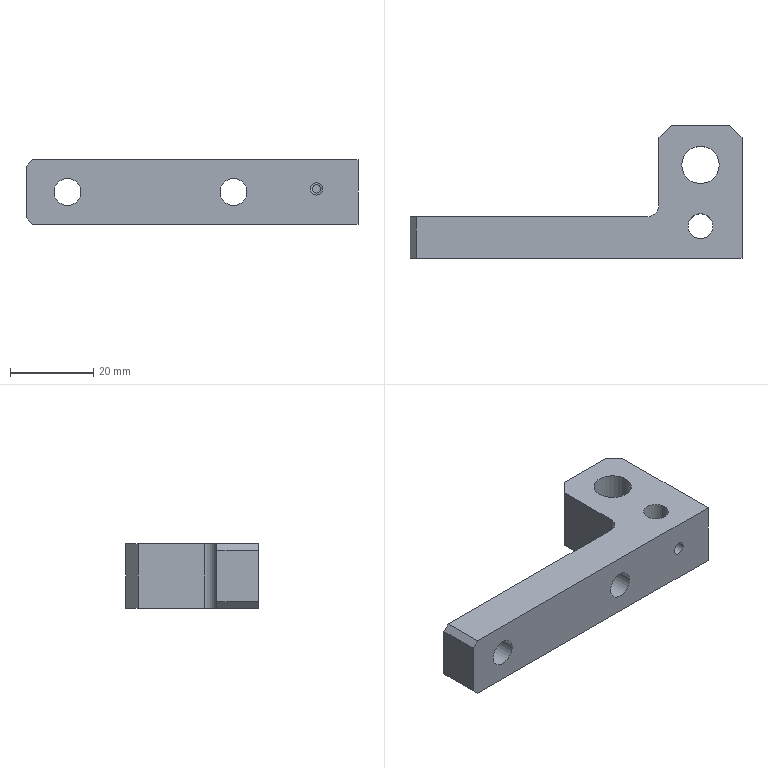Part | NX | 1 solid | 21 faces | box 80 x 32 x 15.5 mm | volume 16646 mm3 | plane 13 | cylinder 8 | commonest cylinder face diameters 6 x2 6.5 x2 2 x1 3 x1 9 x1 12 x1
STEP:
#1=CARTESIAN_POINT('',(70.,18.,9.5));
#2=VERTEX_POINT('',#1);
#3=CARTESIAN_POINT('',(70.784,18.056,9.283));
#4=CARTESIAN_POINT('',(70.,17.972,9.609));
#5=CARTESIAN_POINT('',(69.216,18.056,9.283));
#6=CARTESIAN_POINT('',(68.892,18.141,8.501));
#7=CARTESIAN_POINT('',(69.216,18.056,7.716));
#8=CARTESIAN_POINT('',(70.,17.972,7.392));
#9=CARTESIAN_POINT('',(70.783,18.055,7.716));
#10=CARTESIAN_POINT('',(71.108,18.141,8.499));
#11=CARTESIAN_POINT('',(70.784,18.056,9.283));
#12=CARTESIAN_POINT('',(70.,17.972,9.609));
#13=CARTESIAN_POINT('',(69.216,18.056,9.283));
#14=B_SPLINE_CURVE_WITH_KNOTS('',3,(#3,#4,#5,#6,#7,#8,#9,#10,#11,#12,#13),.UNSPECIFIED.,.T.,.F.,(1,1,1,1,1,1,1,1,1,1,1,1,1,1,1),(-0.002352,-0.001568,-0.000784,0.,0.000784,0.001568,0.002352,0.003136,0.00392,0.004704,0.005488,0.006272,0.007056,0.00784,0.008624),.UNSPECIFIED.);
#15=EDGE_CURVE('',#2,#2,#14,.T.);
#16=ORIENTED_EDGE('',*,*,#15,.T.);
#17=EDGE_LOOP('',(#16));
#18=FACE_BOUND('',#17,.T.);
#19=CARTESIAN_POINT('',(65.5,22.5,15.5));
#20=VERTEX_POINT('',#19);
#21=CARTESIAN_POINT('',(70.,22.5,15.5));
#22=DIRECTION('',(0.,0.,-1.));
#23=DIRECTION('',(-1.,0.,0.));
#24=AXIS2_PLACEMENT_3D('',#21,#22,#23);
#25=CIRCLE('',#24,4.5);
#26=EDGE_CURVE('',#20,#20,#25,.T.);
#27=ORIENTED_EDGE('',*,*,#26,.F.);
#28=EDGE_LOOP('',(#27));
#29=FACE_BOUND('',#28,.T.);
#30=CARTESIAN_POINT('',(65.5,22.5,6.));
#31=VERTEX_POINT('',#30);
#32=CARTESIAN_POINT('',(70.,22.5,6.));
#33=DIRECTION('',(0.,0.,-1.));
#34=DIRECTION('',(-1.,0.,0.));
#35=AXIS2_PLACEMENT_3D('',#32,#33,#34);
#36=CIRCLE('',#35,4.5);
#37=EDGE_CURVE('',#31,#31,#36,.F.);
#38=ORIENTED_EDGE('',*,*,#37,.F.);
#39=EDGE_LOOP('',(#38));
#40=FACE_BOUND('',#39,.T.);
#41=CARTESIAN_POINT('',(70.,22.5,15.5));
#42=DIRECTION('',(0.,0.,-1.));
#43=DIRECTION('',(-1.,0.,0.));
#44=AXIS2_PLACEMENT_3D('',#41,#42,#43);
#45=CYLINDRICAL_SURFACE('',#44,4.5);
#46=ADVANCED_FACE('',(#18,#29,#40),#45,.F.);
#47=ORIENTED_EDGE('',*,*,#26,.T.);
#48=EDGE_LOOP('',(#47));
#49=FACE_BOUND('',#48,.T.);
#50=CARTESIAN_POINT('',(67.,7.75,15.5));
#51=VERTEX_POINT('',#50);
#52=CARTESIAN_POINT('',(70.,7.75,15.5));
#53=DIRECTION('',(0.,0.,-1.));
#54=DIRECTION('',(-1.,0.,0.));
#55=AXIS2_PLACEMENT_3D('',#52,#53,#54);
#56=CIRCLE('',#55,3.);
#57=EDGE_CURVE('',#51,#51,#56,.T.);
#58=ORIENTED_EDGE('',*,*,#57,.T.);
#59=EDGE_LOOP('',(#58));
#60=FACE_BOUND('',#59,.T.);
#61=CARTESIAN_POINT('',(57.,10.,15.5));
#62=VERTEX_POINT('',#61);
#63=CARTESIAN_POINT('',(1.5,10.,15.5));
#64=VERTEX_POINT('',#63);
#65=CARTESIAN_POINT('',(40.,10.,15.5));
#66=DIRECTION('',(-1.,0.,0.));
#67=VECTOR('',#66,1000.);
#68=LINE('',#65,#67);
#69=EDGE_CURVE('',#62,#64,#68,.T.);
#70=ORIENTED_EDGE('',*,*,#69,.T.);
#71=CARTESIAN_POINT('',(1.5,0.,15.5));
#72=VERTEX_POINT('',#71);
#73=CARTESIAN_POINT('',(1.5,16.,15.5));
#74=DIRECTION('',(0.,1.,0.));
#75=VECTOR('',#74,1000.);
#76=LINE('',#73,#75);
#77=EDGE_CURVE('',#64,#72,#76,.F.);
#78=ORIENTED_EDGE('',*,*,#77,.T.);
#79=CARTESIAN_POINT('',(80.,0.,15.5));
#80=VERTEX_POINT('',#79);
#81=CARTESIAN_POINT('',(40.,0.,15.5));
#82=DIRECTION('',(-1.,0.,0.));
#83=VECTOR('',#82,1000.);
#84=LINE('',#81,#83);
#85=EDGE_CURVE('',#80,#72,#84,.T.);
#86=ORIENTED_EDGE('',*,*,#85,.F.);
#87=CARTESIAN_POINT('',(80.,29.,15.5));
#88=VERTEX_POINT('',#87);
#89=CARTESIAN_POINT('',(80.,16.,15.5));
#90=DIRECTION('',(0.,-1.,0.));
#91=VECTOR('',#90,1000.);
#92=LINE('',#89,#91);
#93=EDGE_CURVE('',#88,#80,#92,.T.);
#94=ORIENTED_EDGE('',*,*,#93,.F.);
#95=CARTESIAN_POINT('',(77.,32.,15.5));
#96=VERTEX_POINT('',#95);
#97=CARTESIAN_POINT('',(66.5,42.5,15.5));
#98=DIRECTION('',(0.7071,-0.7071,0.));
#99=VECTOR('',#98,1000.);
#100=LINE('',#97,#99);
#101=EDGE_CURVE('',#88,#96,#100,.F.);
#102=ORIENTED_EDGE('',*,*,#101,.T.);
#103=CARTESIAN_POINT('',(63.,32.,15.5));
#104=VERTEX_POINT('',#103);
#105=CARTESIAN_POINT('',(40.,32.,15.5));
#106=DIRECTION('',(1.,0.,0.));
#107=VECTOR('',#106,1000.);
#108=LINE('',#105,#107);
#109=EDGE_CURVE('',#104,#96,#108,.T.);
#110=ORIENTED_EDGE('',*,*,#109,.F.);
#111=CARTESIAN_POINT('',(60.,29.,15.5));
#112=VERTEX_POINT('',#111);
#113=CARTESIAN_POINT('',(43.5,12.5,15.5));
#114=DIRECTION('',(-0.7071,-0.7071,0.));
#115=VECTOR('',#114,1000.);
#116=LINE('',#113,#115);
#117=EDGE_CURVE('',#104,#112,#116,.T.);
#118=ORIENTED_EDGE('',*,*,#117,.T.);
#119=CARTESIAN_POINT('',(60.,13.,15.5));
#120=VERTEX_POINT('',#119);
#121=CARTESIAN_POINT('',(60.,21.,15.5));
#122=DIRECTION('',(0.,-1.,0.));
#123=VECTOR('',#122,1000.);
#124=LINE('',#121,#123);
#125=EDGE_CURVE('',#112,#120,#124,.T.);
#126=ORIENTED_EDGE('',*,*,#125,.T.);
#127=CARTESIAN_POINT('',(57.,13.,15.5));
#128=DIRECTION('',(0.,0.,1.));
#129=DIRECTION('',(1.,0.,0.));
#130=AXIS2_PLACEMENT_3D('',#127,#128,#129);
#131=CIRCLE('',#130,3.);
#132=EDGE_CURVE('',#120,#62,#131,.F.);
#133=ORIENTED_EDGE('',*,*,#132,.T.);
#134=EDGE_LOOP('',(#70,#78,#86,#94,#102,#110,#118,#126,#133));
#135=FACE_BOUND('',#134,.T.);
#136=CARTESIAN_POINT('',(40.,16.,15.5));
#137=DIRECTION('',(0.,0.,1.));
#138=DIRECTION('',(1.,0.,0.));
#139=AXIS2_PLACEMENT_3D('',#136,#137,#138);
#140=PLANE('',#139);
#141=ADVANCED_FACE('',(#49,#60,#135),#140,.T.);
#142=CARTESIAN_POINT('',(70.,0.,10.));
#143=VERTEX_POINT('',#142);
#144=CARTESIAN_POINT('',(70.,0.,8.5));
#145=DIRECTION('',(0.,1.,0.));
#146=DIRECTION('',(0.,0.,1.));
#147=AXIS2_PLACEMENT_3D('',#144,#145,#146);
#148=CIRCLE('',#147,1.5);
#149=EDGE_CURVE('',#143,#143,#148,.T.);
#150=ORIENTED_EDGE('',*,*,#149,.T.);
#151=EDGE_LOOP('',(#150));
#152=FACE_BOUND('',#151,.T.);
#153=CARTESIAN_POINT('',(50.,0.,11.));
#154=VERTEX_POINT('',#153);
#155=CARTESIAN_POINT('',(50.,0.,7.75));
#156=DIRECTION('',(0.,1.,0.));
#157=DIRECTION('',(0.,0.,1.));
#158=AXIS2_PLACEMENT_3D('',#155,#156,#157);
#159=CIRCLE('',#158,3.25);
#160=EDGE_CURVE('',#154,#154,#159,.T.);
#161=ORIENTED_EDGE('',*,*,#160,.T.);
#162=EDGE_LOOP('',(#161));
#163=FACE_BOUND('',#162,.T.);
#164=CARTESIAN_POINT('',(10.,0.,11.));
#165=VERTEX_POINT('',#164);
#166=CARTESIAN_POINT('',(10.,0.,7.75));
#167=DIRECTION('',(0.,1.,0.));
#168=DIRECTION('',(0.,0.,1.));
#169=AXIS2_PLACEMENT_3D('',#166,#167,#168);
#170=CIRCLE('',#169,3.25);
#171=EDGE_CURVE('',#165,#165,#170,.T.);
#172=ORIENTED_EDGE('',*,*,#171,.T.);
#173=EDGE_LOOP('',(#172));
#174=FACE_BOUND('',#173,.T.);
#175=CARTESIAN_POINT('',(0.,0.,1.5));
#176=VERTEX_POINT('',#175);
#177=CARTESIAN_POINT('',(0.,0.,14.));
#178=VERTEX_POINT('',#177);
#179=CARTESIAN_POINT('',(0.,0.,0.));
#180=DIRECTION('',(0.,0.,1.));
#181=VECTOR('',#180,1000.);
#182=LINE('',#179,#181);
#183=EDGE_CURVE('',#176,#178,#182,.T.);
#184=ORIENTED_EDGE('',*,*,#183,.F.);
#185=CARTESIAN_POINT('',(1.5,0.,0.));
#186=VERTEX_POINT('',#185);
#187=CARTESIAN_POINT('',(20.75,0.,-19.25));
#188=DIRECTION('',(-0.7071,0.,0.7071));
#189=VECTOR('',#188,1000.);
#190=LINE('',#187,#189);
#191=EDGE_CURVE('',#176,#186,#190,.F.);
#192=ORIENTED_EDGE('',*,*,#191,.T.);
#193=CARTESIAN_POINT('',(80.,0.,0.));
#194=VERTEX_POINT('',#193);
#195=CARTESIAN_POINT('',(40.,0.,0.));
#196=DIRECTION('',(1.,0.,0.));
#197=VECTOR('',#196,1000.);
#198=LINE('',#195,#197);
#199=EDGE_CURVE('',#186,#194,#198,.T.);
#200=ORIENTED_EDGE('',*,*,#199,.T.);
#201=CARTESIAN_POINT('',(80.,0.,0.));
#202=DIRECTION('',(0.,0.,1.));
#203=VECTOR('',#202,1000.);
#204=LINE('',#201,#203);
#205=EDGE_CURVE('',#194,#80,#204,.T.);
#206=ORIENTED_EDGE('',*,*,#205,.T.);
#207=ORIENTED_EDGE('',*,*,#85,.T.);
#208=CARTESIAN_POINT('',(13.,0.,27.));
#209=DIRECTION('',(0.7071,0.,0.7071));
#210=VECTOR('',#209,1000.);
#211=LINE('',#208,#210);
#212=EDGE_CURVE('',#72,#178,#211,.F.);
#213=ORIENTED_EDGE('',*,*,#212,.T.);
#214=EDGE_LOOP('',(#184,#192,#200,#206,#207,#213));
#215=FACE_BOUND('',#214,.T.);
#216=CARTESIAN_POINT('',(40.,0.,0.));
#217=DIRECTION('',(0.,-1.,0.));
#218=DIRECTION('',(0.,0.,-1.));
#219=AXIS2_PLACEMENT_3D('',#216,#217,#218);
#220=PLANE('',#219);
#221=ADVANCED_FACE('',(#152,#163,#174,#215),#220,.T.);
#222=CARTESIAN_POINT('',(0.,10.,14.));
#223=VERTEX_POINT('',#222);
#224=CARTESIAN_POINT('',(0.,10.,1.5));
#225=VERTEX_POINT('',#224);
#226=CARTESIAN_POINT('',(0.,10.,0.));
#227=DIRECTION('',(0.,0.,1.));
#228=VECTOR('',#227,1000.);
#229=LINE('',#226,#228);
#230=EDGE_CURVE('',#223,#225,#229,.F.);
#231=ORIENTED_EDGE('',*,*,#230,.T.);
#232=CARTESIAN_POINT('',(0.,16.,1.5));
#233=DIRECTION('',(0.,-1.,0.));
#234=VECTOR('',#233,1000.);
#235=LINE('',#232,#234);
#236=EDGE_CURVE('',#225,#176,#235,.T.);
#237=ORIENTED_EDGE('',*,*,#236,.T.);
#238=ORIENTED_EDGE('',*,*,#183,.T.);
#239=CARTESIAN_POINT('',(0.,16.,14.));
#240=DIRECTION('',(0.,-1.,0.));
#241=VECTOR('',#240,1000.);
#242=LINE('',#239,#241);
#243=EDGE_CURVE('',#178,#223,#242,.F.);
#244=ORIENTED_EDGE('',*,*,#243,.T.);
#245=EDGE_LOOP('',(#231,#237,#238,#244));
#246=FACE_BOUND('',#245,.T.);
#247=CARTESIAN_POINT('',(0.,16.,0.));
#248=DIRECTION('',(-1.,0.,0.));
#249=DIRECTION('',(0.,0.,1.));
#250=AXIS2_PLACEMENT_3D('',#247,#248,#249);
#251=PLANE('',#250);
#252=ADVANCED_FACE('',(#246),#251,.T.);
#253=CARTESIAN_POINT('',(64.,22.5,0.));
#254=VERTEX_POINT('',#253);
#255=CARTESIAN_POINT('',(70.,22.5,0.));
#256=DIRECTION('',(0.,0.,-1.));
#257=DIRECTION('',(-1.,0.,0.));
#258=AXIS2_PLACEMENT_3D('',#255,#256,#257);
#259=CIRCLE('',#258,6.);
#260=EDGE_CURVE('',#254,#254,#259,.T.);
#261=ORIENTED_EDGE('',*,*,#260,.F.);
#262=EDGE_LOOP('',(#261));
#263=FACE_BOUND('',#262,.T.);
#264=CARTESIAN_POINT('',(67.,7.75,0.));
#265=VERTEX_POINT('',#264);
#266=CARTESIAN_POINT('',(70.,7.75,0.));
#267=DIRECTION('',(0.,0.,-1.));
#268=DIRECTION('',(-1.,0.,0.));
#269=AXIS2_PLACEMENT_3D('',#266,#267,#268);
#270=CIRCLE('',#269,3.);
#271=EDGE_CURVE('',#265,#265,#270,.T.);
#272=ORIENTED_EDGE('',*,*,#271,.F.);
#273=EDGE_LOOP('',(#272));
#274=FACE_BOUND('',#273,.T.);
#275=ORIENTED_EDGE('',*,*,#199,.F.);
#276=CARTESIAN_POINT('',(1.5,10.,0.));
#277=VERTEX_POINT('',#276);
#278=CARTESIAN_POINT('',(1.5,16.,0.));
#279=DIRECTION('',(0.,1.,0.));
#280=VECTOR('',#279,1000.);
#281=LINE('',#278,#280);
#282=EDGE_CURVE('',#186,#277,#281,.T.);
#283=ORIENTED_EDGE('',*,*,#282,.T.);
#284=CARTESIAN_POINT('',(57.,10.,0.));
#285=VERTEX_POINT('',#284);
#286=CARTESIAN_POINT('',(40.,10.,0.));
#287=DIRECTION('',(-1.,0.,0.));
#288=VECTOR('',#287,1000.);
#289=LINE('',#286,#288);
#290=EDGE_CURVE('',#277,#285,#289,.F.);
#291=ORIENTED_EDGE('',*,*,#290,.T.);
#292=CARTESIAN_POINT('',(60.,13.,0.));
#293=VERTEX_POINT('',#292);
#294=CARTESIAN_POINT('',(57.,13.,0.));
#295=DIRECTION('',(0.,0.,-1.));
#296=DIRECTION('',(-1.,0.,0.));
#297=AXIS2_PLACEMENT_3D('',#294,#295,#296);
#298=CIRCLE('',#297,3.);
#299=EDGE_CURVE('',#285,#293,#298,.F.);
#300=ORIENTED_EDGE('',*,*,#299,.T.);
#301=CARTESIAN_POINT('',(60.,29.,0.));
#302=VERTEX_POINT('',#301);
#303=CARTESIAN_POINT('',(60.,16.,0.));
#304=DIRECTION('',(0.,-1.,0.));
#305=VECTOR('',#304,1000.);
#306=LINE('',#303,#305);
#307=EDGE_CURVE('',#293,#302,#306,.F.);
#308=ORIENTED_EDGE('',*,*,#307,.T.);
#309=CARTESIAN_POINT('',(63.,32.,0.));
#310=VERTEX_POINT('',#309);
#311=CARTESIAN_POINT('',(43.5,12.5,0.));
#312=DIRECTION('',(0.7071,0.7071,0.));
#313=VECTOR('',#312,1000.);
#314=LINE('',#311,#313);
#315=EDGE_CURVE('',#302,#310,#314,.T.);
#316=ORIENTED_EDGE('',*,*,#315,.T.);
#317=CARTESIAN_POINT('',(77.,32.,0.));
#318=VERTEX_POINT('',#317);
#319=CARTESIAN_POINT('',(40.,32.,0.));
#320=DIRECTION('',(-1.,0.,0.));
#321=VECTOR('',#320,1000.);
#322=LINE('',#319,#321);
#323=EDGE_CURVE('',#318,#310,#322,.T.);
#324=ORIENTED_EDGE('',*,*,#323,.F.);
#325=CARTESIAN_POINT('',(80.,29.,0.));
#326=VERTEX_POINT('',#325);
#327=CARTESIAN_POINT('',(66.5,42.5,0.));
#328=DIRECTION('',(-0.7071,0.7071,0.));
#329=VECTOR('',#328,1000.);
#330=LINE('',#327,#329);
#331=EDGE_CURVE('',#318,#326,#330,.F.);
#332=ORIENTED_EDGE('',*,*,#331,.T.);
#333=CARTESIAN_POINT('',(80.,16.,0.));
#334=DIRECTION('',(0.,1.,0.));
#335=VECTOR('',#334,1000.);
#336=LINE('',#333,#335);
#337=EDGE_CURVE('',#194,#326,#336,.T.);
#338=ORIENTED_EDGE('',*,*,#337,.F.);
#339=EDGE_LOOP('',(#275,#283,#291,#300,#308,#316,#324,#332,#338));
#340=FACE_BOUND('',#339,.T.);
#341=CARTESIAN_POINT('',(40.,16.,0.));
#342=DIRECTION('',(0.,0.,-1.));
#343=DIRECTION('',(-1.,0.,0.));
#344=AXIS2_PLACEMENT_3D('',#341,#342,#343);
#345=PLANE('',#344);
#346=ADVANCED_FACE('',(#263,#274,#340),#345,.T.);
#347=ORIENTED_EDGE('',*,*,#337,.T.);
#348=CARTESIAN_POINT('',(80.,29.,0.));
#349=DIRECTION('',(0.,0.,1.));
#350=VECTOR('',#349,1000.);
#351=LINE('',#348,#350);
#352=EDGE_CURVE('',#326,#88,#351,.T.);
#353=ORIENTED_EDGE('',*,*,#352,.T.);
#354=ORIENTED_EDGE('',*,*,#93,.T.);
#355=ORIENTED_EDGE('',*,*,#205,.F.);
#356=EDGE_LOOP('',(#347,#353,#354,#355));
#357=FACE_BOUND('',#356,.T.);
#358=CARTESIAN_POINT('',(80.,16.,0.));
#359=DIRECTION('',(1.,0.,0.));
#360=DIRECTION('',(0.,0.,-1.));
#361=AXIS2_PLACEMENT_3D('',#358,#359,#360);
#362=PLANE('',#361);
#363=ADVANCED_FACE('',(#357),#362,.T.);
#364=CARTESIAN_POINT('',(50.,10.,4.5));
#365=VERTEX_POINT('',#364);
#366=CARTESIAN_POINT('',(50.,10.,7.75));
#367=DIRECTION('',(0.,-1.,0.));
#368=DIRECTION('',(0.,0.,-1.));
#369=AXIS2_PLACEMENT_3D('',#366,#367,#368);
#370=CIRCLE('',#369,3.25);
#371=EDGE_CURVE('',#365,#365,#370,.T.);
#372=ORIENTED_EDGE('',*,*,#371,.T.);
#373=EDGE_LOOP('',(#372));
#374=FACE_BOUND('',#373,.T.);
#375=CARTESIAN_POINT('',(10.,10.,4.5));
#376=VERTEX_POINT('',#375);
#377=CARTESIAN_POINT('',(10.,10.,7.75));
#378=DIRECTION('',(0.,-1.,0.));
#379=DIRECTION('',(0.,0.,-1.));
#380=AXIS2_PLACEMENT_3D('',#377,#378,#379);
#381=CIRCLE('',#380,3.25);
#382=EDGE_CURVE('',#376,#376,#381,.T.);
#383=ORIENTED_EDGE('',*,*,#382,.T.);
#384=EDGE_LOOP('',(#383));
#385=FACE_BOUND('',#384,.T.);
#386=ORIENTED_EDGE('',*,*,#290,.F.);
#387=CARTESIAN_POINT('',(0.,10.,1.5));
#388=DIRECTION('',(0.7071,0.,-0.7071));
#389=VECTOR('',#388,1000.);
#390=LINE('',#387,#389);
#391=EDGE_CURVE('',#277,#225,#390,.F.);
#392=ORIENTED_EDGE('',*,*,#391,.T.);
#393=ORIENTED_EDGE('',*,*,#230,.F.);
#394=CARTESIAN_POINT('',(0.,10.,14.));
#395=DIRECTION('',(-0.7071,0.,-0.7071));
#396=VECTOR('',#395,1000.);
#397=LINE('',#394,#396);
#398=EDGE_CURVE('',#223,#64,#397,.F.);
#399=ORIENTED_EDGE('',*,*,#398,.T.);
#400=ORIENTED_EDGE('',*,*,#69,.F.);
#401=CARTESIAN_POINT('',(57.,10.,0.));
#402=DIRECTION('',(0.,0.,-1.));
#403=VECTOR('',#402,1000.);
#404=LINE('',#401,#403);
#405=EDGE_CURVE('',#62,#285,#404,.T.);
#406=ORIENTED_EDGE('',*,*,#405,.T.);
#407=EDGE_LOOP('',(#386,#392,#393,#399,#400,#406));
#408=FACE_BOUND('',#407,.T.);
#409=CARTESIAN_POINT('',(40.,10.,6.));
#410=DIRECTION('',(0.,-1.,0.));
#411=DIRECTION('',(0.,0.,-1.));
#412=AXIS2_PLACEMENT_3D('',#409,#410,#411);
#413=PLANE('',#412);
#414=ADVANCED_FACE('',(#374,#385,#408),#413,.F.);
#415=ORIENTED_EDGE('',*,*,#109,.T.);
#416=CARTESIAN_POINT('',(77.,32.,0.));
#417=DIRECTION('',(0.,0.,-1.));
#418=VECTOR('',#417,1000.);
#419=LINE('',#416,#418);
#420=EDGE_CURVE('',#96,#318,#419,.T.);
#421=ORIENTED_EDGE('',*,*,#420,.T.);
#422=ORIENTED_EDGE('',*,*,#323,.T.);
#423=CARTESIAN_POINT('',(63.,32.,12.));
#424=DIRECTION('',(0.,0.,1.));
#425=VECTOR('',#424,1000.);
#426=LINE('',#423,#425);
#427=EDGE_CURVE('',#310,#104,#426,.T.);
#428=ORIENTED_EDGE('',*,*,#427,.T.);
#429=EDGE_LOOP('',(#415,#421,#422,#428));
#430=FACE_BOUND('',#429,.T.);
#431=CARTESIAN_POINT('',(40.,32.,0.));
#432=DIRECTION('',(0.,1.,0.));
#433=DIRECTION('',(0.,0.,1.));
#434=AXIS2_PLACEMENT_3D('',#431,#432,#433);
#435=PLANE('',#434);
#436=ADVANCED_FACE('',(#430),#435,.T.);
#437=ORIENTED_EDGE('',*,*,#125,.F.);
#438=CARTESIAN_POINT('',(60.,29.,0.));
#439=DIRECTION('',(0.,0.,-1.));
#440=VECTOR('',#439,1000.);
#441=LINE('',#438,#440);
#442=EDGE_CURVE('',#112,#302,#441,.T.);
#443=ORIENTED_EDGE('',*,*,#442,.T.);
#444=ORIENTED_EDGE('',*,*,#307,.F.);
#445=CARTESIAN_POINT('',(60.,13.,12.));
#446=DIRECTION('',(0.,0.,-1.));
#447=VECTOR('',#446,1000.);
#448=LINE('',#445,#447);
#449=EDGE_CURVE('',#293,#120,#448,.F.);
#450=ORIENTED_EDGE('',*,*,#449,.T.);
#451=EDGE_LOOP('',(#437,#443,#444,#450));
#452=FACE_BOUND('',#451,.T.);
#453=CARTESIAN_POINT('',(60.,21.,6.));
#454=DIRECTION('',(1.,0.,0.));
#455=DIRECTION('',(0.,0.,-1.));
#456=AXIS2_PLACEMENT_3D('',#453,#454,#455);
#457=PLANE('',#456);
#458=ADVANCED_FACE('',(#452),#457,.F.);
#459=ORIENTED_EDGE('',*,*,#132,.F.);
#460=ORIENTED_EDGE('',*,*,#449,.F.);
#461=ORIENTED_EDGE('',*,*,#299,.F.);
#462=ORIENTED_EDGE('',*,*,#405,.F.);
#463=EDGE_LOOP('',(#459,#460,#461,#462));
#464=FACE_BOUND('',#463,.T.);
#465=CARTESIAN_POINT('',(57.,13.,6.));
#466=DIRECTION('',(0.,0.,1.));
#467=DIRECTION('',(1.,0.,0.));
#468=AXIS2_PLACEMENT_3D('',#465,#466,#467);
#469=CYLINDRICAL_SURFACE('',#468,3.);
#470=ADVANCED_FACE('',(#464),#469,.F.);
#471=ORIENTED_EDGE('',*,*,#331,.F.);
#472=ORIENTED_EDGE('',*,*,#420,.F.);
#473=ORIENTED_EDGE('',*,*,#101,.F.);
#474=ORIENTED_EDGE('',*,*,#352,.F.);
#475=EDGE_LOOP('',(#471,#472,#473,#474));
#476=FACE_BOUND('',#475,.T.);
#477=CARTESIAN_POINT('',(80.,29.,0.));
#478=DIRECTION('',(-0.7071,-0.7071,0.));
#479=DIRECTION('',(0.,0.,1.));
#480=AXIS2_PLACEMENT_3D('',#477,#478,#479);
#481=PLANE('',#480);
#482=ADVANCED_FACE('',(#476),#481,.F.);
#483=ORIENTED_EDGE('',*,*,#117,.F.);
#484=ORIENTED_EDGE('',*,*,#427,.F.);
#485=ORIENTED_EDGE('',*,*,#315,.F.);
#486=ORIENTED_EDGE('',*,*,#442,.F.);
#487=EDGE_LOOP('',(#483,#484,#485,#486));
#488=FACE_BOUND('',#487,.T.);
#489=CARTESIAN_POINT('',(60.,29.,6.));
#490=DIRECTION('',(-0.7071,0.7071,0.));
#491=DIRECTION('',(0.,0.,1.));
#492=AXIS2_PLACEMENT_3D('',#489,#490,#491);
#493=PLANE('',#492);
#494=ADVANCED_FACE('',(#488),#493,.T.);
#495=ORIENTED_EDGE('',*,*,#391,.F.);
#496=ORIENTED_EDGE('',*,*,#282,.F.);
#497=ORIENTED_EDGE('',*,*,#191,.F.);
#498=ORIENTED_EDGE('',*,*,#236,.F.);
#499=EDGE_LOOP('',(#495,#496,#497,#498));
#500=FACE_BOUND('',#499,.T.);
#501=CARTESIAN_POINT('',(0.,16.,1.5));
#502=DIRECTION('',(0.7071,0.,0.7071));
#503=DIRECTION('',(0.,-1.,0.));
#504=AXIS2_PLACEMENT_3D('',#501,#502,#503);
#505=PLANE('',#504);
#506=ADVANCED_FACE('',(#500),#505,.F.);
#507=ORIENTED_EDGE('',*,*,#212,.F.);
#508=ORIENTED_EDGE('',*,*,#77,.F.);
#509=ORIENTED_EDGE('',*,*,#398,.F.);
#510=ORIENTED_EDGE('',*,*,#243,.F.);
#511=EDGE_LOOP('',(#507,#508,#509,#510));
#512=FACE_BOUND('',#511,.T.);
#513=CARTESIAN_POINT('',(0.,16.,14.));
#514=DIRECTION('',(0.7071,0.,-0.7071));
#515=DIRECTION('',(-0.7071,0.,-0.7071));
#516=AXIS2_PLACEMENT_3D('',#513,#514,#515);
#517=PLANE('',#516);
#518=ADVANCED_FACE('',(#512),#517,.F.);
#519=ORIENTED_EDGE('',*,*,#171,.F.);
#520=EDGE_LOOP('',(#519));
#521=FACE_BOUND('',#520,.T.);
#522=ORIENTED_EDGE('',*,*,#382,.F.);
#523=EDGE_LOOP('',(#522));
#524=FACE_BOUND('',#523,.T.);
#525=CARTESIAN_POINT('',(10.,0.,7.75));
#526=DIRECTION('',(0.,1.,0.));
#527=DIRECTION('',(0.,0.,1.));
#528=AXIS2_PLACEMENT_3D('',#525,#526,#527);
#529=CYLINDRICAL_SURFACE('',#528,3.25);
#530=ADVANCED_FACE('',(#521,#524),#529,.F.);
#531=ORIENTED_EDGE('',*,*,#160,.F.);
#532=EDGE_LOOP('',(#531));
#533=FACE_BOUND('',#532,.T.);
#534=ORIENTED_EDGE('',*,*,#371,.F.);
#535=EDGE_LOOP('',(#534));
#536=FACE_BOUND('',#535,.T.);
#537=CARTESIAN_POINT('',(50.,0.,7.75));
#538=DIRECTION('',(0.,1.,0.));
#539=DIRECTION('',(0.,0.,1.));
#540=AXIS2_PLACEMENT_3D('',#537,#538,#539);
#541=CYLINDRICAL_SURFACE('',#540,3.25);
#542=ADVANCED_FACE('',(#533,#536),#541,.F.);
#543=CARTESIAN_POINT('',(70.,4.75,10.));
#544=VERTEX_POINT('',#543);
#545=CARTESIAN_POINT('',(71.178,4.938,9.674));
#546=CARTESIAN_POINT('',(69.999,4.656,10.163));
#547=CARTESIAN_POINT('',(68.824,4.937,9.673));
#548=CARTESIAN_POINT('',(68.338,5.259,8.505));
#549=CARTESIAN_POINT('',(68.823,4.938,7.327));
#550=CARTESIAN_POINT('',(69.994,4.656,6.837));
#551=CARTESIAN_POINT('',(71.176,4.936,7.325));
#552=CARTESIAN_POINT('',(71.661,5.259,8.495));
#553=CARTESIAN_POINT('',(71.178,4.938,9.674));
#554=CARTESIAN_POINT('',(69.999,4.656,10.163));
#555=CARTESIAN_POINT('',(68.824,4.937,9.673));
#556=B_SPLINE_CURVE_WITH_KNOTS('',3,(#545,#546,#547,#548,#549,#550,#551,#552,#553,#554,#555),.UNSPECIFIED.,.T.,.F.,(1,1,1,1,1,1,1,1,1,1,1,1,1,1,1),(-0.003575,-0.002384,-0.001192,0.,0.001192,0.002384,0.003575,0.004767,0.005959,0.007151,0.008343,0.009535,0.01073,0.01192,0.01311),.UNSPECIFIED.);
#557=EDGE_CURVE('',#544,#544,#556,.T.);
#558=ORIENTED_EDGE('',*,*,#557,.T.);
#559=EDGE_LOOP('',(#558));
#560=FACE_BOUND('',#559,.T.);
#561=CARTESIAN_POINT('',(70.,10.75,9.5));
#562=VERTEX_POINT('',#561);
#563=CARTESIAN_POINT('',(69.216,10.667,9.283));
#564=CARTESIAN_POINT('',(70.,10.792,9.608));
#565=CARTESIAN_POINT('',(70.784,10.667,9.283));
#566=CARTESIAN_POINT('',(71.108,10.534,8.501));
#567=CARTESIAN_POINT('',(70.783,10.667,7.716));
#568=CARTESIAN_POINT('',(70.001,10.792,7.392));
#569=CARTESIAN_POINT('',(69.216,10.667,7.716));
#570=CARTESIAN_POINT('',(68.892,10.534,8.5));
#571=CARTESIAN_POINT('',(69.216,10.667,9.283));
#572=CARTESIAN_POINT('',(70.,10.792,9.608));
#573=CARTESIAN_POINT('',(70.784,10.667,9.283));
#574=B_SPLINE_CURVE_WITH_KNOTS('',3,(#563,#564,#565,#566,#567,#568,#569,#570,#571,#572,#573),.UNSPECIFIED.,.T.,.F.,(1,1,1,1,1,1,1,1,1,1,1,1,1,1,1),(-0.002362,-0.001574,-0.0007872,0.,0.0007872,0.001574,0.002362,0.003149,0.003936,0.004723,0.00551,0.006298,0.007085,0.007872,0.008659),.UNSPECIFIED.);
#575=EDGE_CURVE('',#562,#562,#574,.T.);
#576=ORIENTED_EDGE('',*,*,#575,.T.);
#577=EDGE_LOOP('',(#576));
#578=FACE_BOUND('',#577,.T.);
#579=ORIENTED_EDGE('',*,*,#271,.T.);
#580=EDGE_LOOP('',(#579));
#581=FACE_BOUND('',#580,.T.);
#582=ORIENTED_EDGE('',*,*,#57,.F.);
#583=EDGE_LOOP('',(#582));
#584=FACE_BOUND('',#583,.T.);
#585=CARTESIAN_POINT('',(70.,7.75,15.5));
#586=DIRECTION('',(0.,0.,-1.));
#587=DIRECTION('',(-1.,0.,0.));
#588=AXIS2_PLACEMENT_3D('',#585,#586,#587);
#589=CYLINDRICAL_SURFACE('',#588,3.);
#590=ADVANCED_FACE('',(#560,#578,#581,#584),#589,.F.);
#591=CARTESIAN_POINT('',(64.,22.5,6.));
#592=VERTEX_POINT('',#591);
#593=CARTESIAN_POINT('',(70.,22.5,6.));
#594=DIRECTION('',(0.,0.,-1.));
#595=DIRECTION('',(-1.,0.,0.));
#596=AXIS2_PLACEMENT_3D('',#593,#594,#595);
#597=CIRCLE('',#596,6.);
#598=EDGE_CURVE('',#592,#592,#597,.F.);
#599=ORIENTED_EDGE('',*,*,#598,.F.);
#600=EDGE_LOOP('',(#599));
#601=FACE_BOUND('',#600,.T.);
#602=ORIENTED_EDGE('',*,*,#37,.T.);
#603=EDGE_LOOP('',(#602));
#604=FACE_BOUND('',#603,.T.);
#605=CARTESIAN_POINT('',(70.,22.5,6.));
#606=DIRECTION('',(0.,0.,-1.));
#607=DIRECTION('',(-1.,0.,0.));
#608=AXIS2_PLACEMENT_3D('',#605,#606,#607);
#609=PLANE('',#608);
#610=ADVANCED_FACE('',(#601,#604),#609,.T.);
#611=ORIENTED_EDGE('',*,*,#260,.T.);
#612=EDGE_LOOP('',(#611));
#613=FACE_BOUND('',#612,.T.);
#614=ORIENTED_EDGE('',*,*,#598,.T.);
#615=EDGE_LOOP('',(#614));
#616=FACE_BOUND('',#615,.T.);
#617=CARTESIAN_POINT('',(70.,22.5,6.));
#618=DIRECTION('',(0.,0.,-1.));
#619=DIRECTION('',(-1.,0.,0.));
#620=AXIS2_PLACEMENT_3D('',#617,#618,#619);
#621=CYLINDRICAL_SURFACE('',#620,6.);
#622=ADVANCED_FACE('',(#613,#616),#621,.F.);
#623=ORIENTED_EDGE('',*,*,#575,.F.);
#624=EDGE_LOOP('',(#623));
#625=FACE_BOUND('',#624,.T.);
#626=ORIENTED_EDGE('',*,*,#15,.F.);
#627=EDGE_LOOP('',(#626));
#628=FACE_BOUND('',#627,.T.);
#629=CARTESIAN_POINT('',(70.,0.,8.5));
#630=DIRECTION('',(0.,1.,0.));
#631=DIRECTION('',(0.,0.,1.));
#632=AXIS2_PLACEMENT_3D('',#629,#630,#631);
#633=CYLINDRICAL_SURFACE('',#632,1.);
#634=ADVANCED_FACE('',(#625,#628),#633,.F.);
#635=ORIENTED_EDGE('',*,*,#149,.F.);
#636=EDGE_LOOP('',(#635));
#637=FACE_BOUND('',#636,.T.);
#638=ORIENTED_EDGE('',*,*,#557,.F.);
#639=EDGE_LOOP('',(#638));
#640=FACE_BOUND('',#639,.T.);
#641=CARTESIAN_POINT('',(70.,0.,8.5));
#642=DIRECTION('',(0.,1.,0.));
#643=DIRECTION('',(0.,0.,1.));
#644=AXIS2_PLACEMENT_3D('',#641,#642,#643);
#645=CYLINDRICAL_SURFACE('',#644,1.5);
#646=ADVANCED_FACE('',(#637,#640),#645,.F.);
#647=CLOSED_SHELL('',(#46,#141,#221,#252,#346,#363,#414,#436,#458,#470,#482,#494,#506,#518,#530,#542,#590,#610,#622,#634,#646));
#648=MANIFOLD_SOLID_BREP('',#647);
#649=(LENGTH_UNIT()NAMED_UNIT(*)SI_UNIT(.MILLI.,.METRE.));
#650=UNCERTAINTY_MEASURE_WITH_UNIT(LENGTH_MEASURE(0.0508),#649,'','');
#651=(NAMED_UNIT(*)PLANE_ANGLE_UNIT()SI_UNIT($,.RADIAN.));
#652=(NAMED_UNIT(*)SI_UNIT($,.STERADIAN.)SOLID_ANGLE_UNIT());
#653=(GEOMETRIC_REPRESENTATION_CONTEXT(3)GLOBAL_UNCERTAINTY_ASSIGNED_CONTEXT((#650))GLOBAL_UNIT_ASSIGNED_CONTEXT((#649,#651,#652))REPRESENTATION_CONTEXT('',''));
#654=ADVANCED_BREP_SHAPE_REPRESENTATION('',(#648),#653);